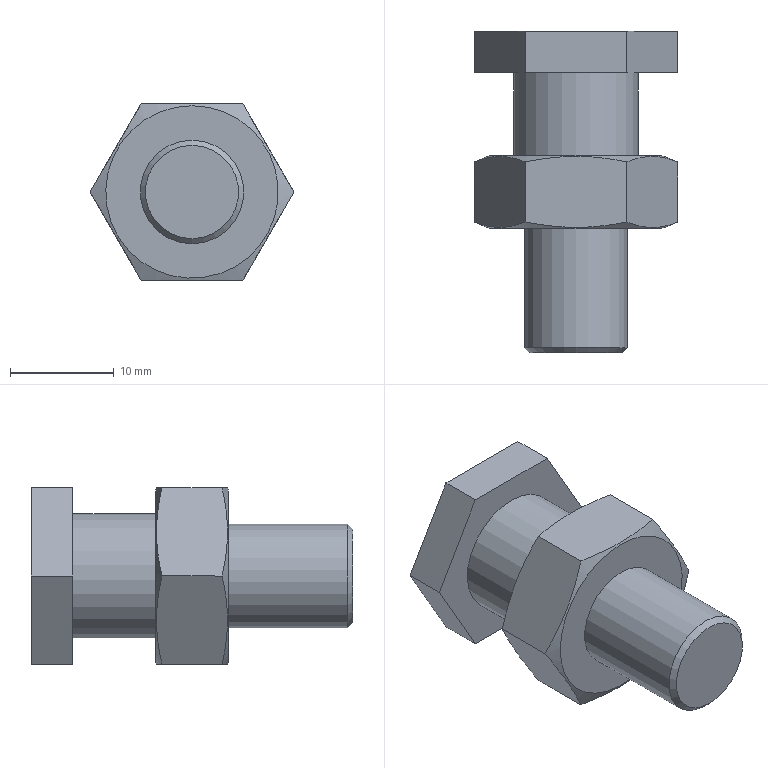Part | NX | 1 solid | 22 faces | box 19.63 x 31 x 17 mm | volume 4585 mm3 | plane 17 | cone 3 | cylinder 2 | commonest cylinder face diameters 10 x1 12 x1
STEP:
#1=CARTESIAN_POINT('',(0.,-7.,8.315));
#2=VERTEX_POINT('',#1);
#3=CARTESIAN_POINT('',(0.,-7.,0.));
#4=DIRECTION('',(0.,1.,0.));
#5=DIRECTION('',(0.,0.,1.));
#6=AXIS2_PLACEMENT_3D('',#3,#4,#5);
#7=CIRCLE('',#6,8.315);
#8=EDGE_CURVE('',#2,#2,#7,.T.);
#9=ORIENTED_EDGE('',*,*,#8,.F.);
#10=EDGE_LOOP('',(#9));
#11=FACE_BOUND('',#10,.T.);
#12=CARTESIAN_POINT('',(0.,-7.,5.));
#13=VERTEX_POINT('',#12);
#14=CARTESIAN_POINT('',(0.,-7.,0.));
#15=DIRECTION('',(0.,1.,0.));
#16=DIRECTION('',(0.,0.,1.));
#17=AXIS2_PLACEMENT_3D('',#14,#15,#16);
#18=CIRCLE('',#17,5.);
#19=EDGE_CURVE('',#13,#13,#18,.F.);
#20=ORIENTED_EDGE('',*,*,#19,.F.);
#21=EDGE_LOOP('',(#20));
#22=FACE_BOUND('',#21,.T.);
#23=CARTESIAN_POINT('',(0.,-7.,0.));
#24=DIRECTION('',(0.,1.,0.));
#25=DIRECTION('',(0.,0.,1.));
#26=AXIS2_PLACEMENT_3D('',#23,#24,#25);
#27=PLANE('',#26);
#28=ADVANCED_FACE('',(#11,#22),#27,.F.);
#29=CARTESIAN_POINT('',(4.907,-6.4,8.5));
#30=VERTEX_POINT('',#29);
#31=CARTESIAN_POINT('',(4.907,-0.6,8.5));
#32=VERTEX_POINT('',#31);
#33=CARTESIAN_POINT('',(4.907,-7.,8.5));
#34=DIRECTION('',(0.,1.,0.));
#35=VECTOR('',#34,1000.);
#36=LINE('',#33,#35);
#37=EDGE_CURVE('',#30,#32,#36,.T.);
#38=ORIENTED_EDGE('',*,*,#37,.F.);
#39=CARTESIAN_POINT('',(9.815,-6.4,0.));
#40=VERTEX_POINT('',#39);
#41=CARTESIAN_POINT('',(4.907,-6.4,8.5));
#42=CARTESIAN_POINT('',(5.721,-6.725,7.091));
#43=CARTESIAN_POINT('',(7.35,-7.126,4.27));
#44=CARTESIAN_POINT('',(9.,-6.726,1.412));
#45=CARTESIAN_POINT('',(9.815,-6.4,0.));
#46=B_SPLINE_CURVE_WITH_KNOTS('',3,(#41,#42,#43,#44,#45),.UNSPECIFIED.,.F.,.F.,(4,1,4),(0.000000232,0.004909,0.009818),.UNSPECIFIED.);
#47=EDGE_CURVE('',#30,#40,#46,.T.);
#48=ORIENTED_EDGE('',*,*,#47,.T.);
#49=CARTESIAN_POINT('',(9.815,-0.6,0.));
#50=VERTEX_POINT('',#49);
#51=CARTESIAN_POINT('',(9.815,-7.,0.));
#52=DIRECTION('',(0.,1.,0.));
#53=VECTOR('',#52,1000.);
#54=LINE('',#51,#53);
#55=EDGE_CURVE('',#40,#50,#54,.T.);
#56=ORIENTED_EDGE('',*,*,#55,.T.);
#57=CARTESIAN_POINT('',(9.815,-0.6,0.));
#58=CARTESIAN_POINT('',(9.001,-0.2746,1.409));
#59=CARTESIAN_POINT('',(7.373,0.1262,4.23));
#60=CARTESIAN_POINT('',(5.723,-0.2738,7.088));
#61=CARTESIAN_POINT('',(4.907,-0.6,8.5));
#62=B_SPLINE_CURVE_WITH_KNOTS('',3,(#57,#58,#59,#60,#61),.UNSPECIFIED.,.F.,.F.,(4,1,4),(0.000000232,0.004909,0.009818),.UNSPECIFIED.);
#63=EDGE_CURVE('',#50,#32,#62,.T.);
#64=ORIENTED_EDGE('',*,*,#63,.T.);
#65=EDGE_LOOP('',(#38,#48,#56,#64));
#66=FACE_BOUND('',#65,.T.);
#67=CARTESIAN_POINT('',(4.907,-7.,8.5));
#68=DIRECTION('',(0.866,0.,0.5));
#69=DIRECTION('',(0.5,0.,-0.866));
#70=AXIS2_PLACEMENT_3D('',#67,#68,#69);
#71=PLANE('',#70);
#72=ADVANCED_FACE('',(#66),#71,.T.);
#73=CARTESIAN_POINT('',(-4.907,-6.4,8.5));
#74=VERTEX_POINT('',#73);
#75=CARTESIAN_POINT('',(-4.907,-0.6,8.5));
#76=VERTEX_POINT('',#75);
#77=CARTESIAN_POINT('',(-4.907,-7.,8.5));
#78=DIRECTION('',(0.,1.,0.));
#79=VECTOR('',#78,1000.);
#80=LINE('',#77,#79);
#81=EDGE_CURVE('',#74,#76,#80,.T.);
#82=ORIENTED_EDGE('',*,*,#81,.F.);
#83=CARTESIAN_POINT('',(-4.907,-6.4,8.5));
#84=CARTESIAN_POINT('',(-3.285,-6.724,8.5));
#85=CARTESIAN_POINT('',(0.004586,-7.128,8.5));
#86=CARTESIAN_POINT('',(3.286,-6.724,8.5));
#87=CARTESIAN_POINT('',(4.907,-6.4,8.5));
#88=B_SPLINE_CURVE_WITH_KNOTS('',3,(#83,#84,#85,#86,#87),.UNSPECIFIED.,.F.,.F.,(4,1,4),(0.0084,0.01335,0.01831),.UNSPECIFIED.);
#89=EDGE_CURVE('',#74,#30,#88,.T.);
#90=ORIENTED_EDGE('',*,*,#89,.T.);
#91=ORIENTED_EDGE('',*,*,#37,.T.);
#92=CARTESIAN_POINT('',(-4.907,-0.6,8.5));
#93=CARTESIAN_POINT('',(-3.285,-0.2755,8.5));
#94=CARTESIAN_POINT('',(0.004586,0.1276,8.5));
#95=CARTESIAN_POINT('',(3.286,-0.2757,8.5));
#96=CARTESIAN_POINT('',(4.907,-0.6,8.5));
#97=B_SPLINE_CURVE_WITH_KNOTS('',3,(#92,#93,#94,#95,#96),.UNSPECIFIED.,.F.,.F.,(4,1,4),(0.0084,0.01335,0.01831),.UNSPECIFIED.);
#98=EDGE_CURVE('',#32,#76,#97,.F.);
#99=ORIENTED_EDGE('',*,*,#98,.T.);
#100=EDGE_LOOP('',(#82,#90,#91,#99));
#101=FACE_BOUND('',#100,.T.);
#102=CARTESIAN_POINT('',(-4.907,-7.,8.5));
#103=DIRECTION('',(0.,0.,1.));
#104=DIRECTION('',(1.,0.,0.));
#105=AXIS2_PLACEMENT_3D('',#102,#103,#104);
#106=PLANE('',#105);
#107=ADVANCED_FACE('',(#101),#106,.T.);
#108=CARTESIAN_POINT('',(-9.815,-6.4,0.));
#109=VERTEX_POINT('',#108);
#110=CARTESIAN_POINT('',(-9.815,-0.6,0.));
#111=VERTEX_POINT('',#110);
#112=CARTESIAN_POINT('',(-9.815,-7.,0.));
#113=DIRECTION('',(0.,1.,0.));
#114=VECTOR('',#113,1000.);
#115=LINE('',#112,#114);
#116=EDGE_CURVE('',#109,#111,#115,.T.);
#117=ORIENTED_EDGE('',*,*,#116,.F.);
#118=CARTESIAN_POINT('',(-9.815,-6.4,0.));
#119=CARTESIAN_POINT('',(-9.001,-6.725,1.409));
#120=CARTESIAN_POINT('',(-7.373,-7.126,4.23));
#121=CARTESIAN_POINT('',(-5.723,-6.726,7.088));
#122=CARTESIAN_POINT('',(-4.907,-6.4,8.5));
#123=B_SPLINE_CURVE_WITH_KNOTS('',3,(#118,#119,#120,#121,#122),.UNSPECIFIED.,.F.,.F.,(4,1,4),(0.000000232,0.004909,0.009818),.UNSPECIFIED.);
#124=EDGE_CURVE('',#109,#74,#123,.T.);
#125=ORIENTED_EDGE('',*,*,#124,.T.);
#126=ORIENTED_EDGE('',*,*,#81,.T.);
#127=CARTESIAN_POINT('',(-4.907,-0.6,8.5));
#128=CARTESIAN_POINT('',(-5.721,-0.2746,7.091));
#129=CARTESIAN_POINT('',(-7.35,0.1262,4.27));
#130=CARTESIAN_POINT('',(-9.,-0.2738,1.412));
#131=CARTESIAN_POINT('',(-9.815,-0.6,0.));
#132=B_SPLINE_CURVE_WITH_KNOTS('',3,(#127,#128,#129,#130,#131),.UNSPECIFIED.,.F.,.F.,(4,1,4),(0.000000232,0.004909,0.009818),.UNSPECIFIED.);
#133=EDGE_CURVE('',#76,#111,#132,.T.);
#134=ORIENTED_EDGE('',*,*,#133,.T.);
#135=EDGE_LOOP('',(#117,#125,#126,#134));
#136=FACE_BOUND('',#135,.T.);
#137=CARTESIAN_POINT('',(-9.815,-7.,0.));
#138=DIRECTION('',(-0.866,0.,0.5));
#139=DIRECTION('',(0.5,0.,0.866));
#140=AXIS2_PLACEMENT_3D('',#137,#138,#139);
#141=PLANE('',#140);
#142=ADVANCED_FACE('',(#136),#141,.T.);
#143=CARTESIAN_POINT('',(-4.907,-6.4,-8.5));
#144=VERTEX_POINT('',#143);
#145=CARTESIAN_POINT('',(-4.907,-0.6,-8.5));
#146=VERTEX_POINT('',#145);
#147=CARTESIAN_POINT('',(-4.907,-7.,-8.5));
#148=DIRECTION('',(0.,1.,0.));
#149=VECTOR('',#148,1000.);
#150=LINE('',#147,#149);
#151=EDGE_CURVE('',#144,#146,#150,.T.);
#152=ORIENTED_EDGE('',*,*,#151,.F.);
#153=CARTESIAN_POINT('',(-4.907,-6.4,-8.5));
#154=CARTESIAN_POINT('',(-5.721,-6.725,-7.091));
#155=CARTESIAN_POINT('',(-7.35,-7.126,-4.27));
#156=CARTESIAN_POINT('',(-9.,-6.726,-1.412));
#157=CARTESIAN_POINT('',(-9.815,-6.4,0.));
#158=B_SPLINE_CURVE_WITH_KNOTS('',3,(#153,#154,#155,#156,#157),.UNSPECIFIED.,.F.,.F.,(4,1,4),(0.000000232,0.004909,0.009818),.UNSPECIFIED.);
#159=EDGE_CURVE('',#144,#109,#158,.T.);
#160=ORIENTED_EDGE('',*,*,#159,.T.);
#161=ORIENTED_EDGE('',*,*,#116,.T.);
#162=CARTESIAN_POINT('',(-9.815,-0.6,0.));
#163=CARTESIAN_POINT('',(-9.001,-0.2746,-1.409));
#164=CARTESIAN_POINT('',(-7.373,0.1262,-4.23));
#165=CARTESIAN_POINT('',(-5.723,-0.2738,-7.088));
#166=CARTESIAN_POINT('',(-4.907,-0.6,-8.5));
#167=B_SPLINE_CURVE_WITH_KNOTS('',3,(#162,#163,#164,#165,#166),.UNSPECIFIED.,.F.,.F.,(4,1,4),(0.000000232,0.004909,0.009818),.UNSPECIFIED.);
#168=EDGE_CURVE('',#111,#146,#167,.T.);
#169=ORIENTED_EDGE('',*,*,#168,.T.);
#170=EDGE_LOOP('',(#152,#160,#161,#169));
#171=FACE_BOUND('',#170,.T.);
#172=CARTESIAN_POINT('',(-4.907,-7.,-8.5));
#173=DIRECTION('',(-0.866,0.,-0.5));
#174=DIRECTION('',(-0.5,0.,0.866));
#175=AXIS2_PLACEMENT_3D('',#172,#173,#174);
#176=PLANE('',#175);
#177=ADVANCED_FACE('',(#171),#176,.T.);
#178=CARTESIAN_POINT('',(4.907,-6.4,-8.5));
#179=VERTEX_POINT('',#178);
#180=CARTESIAN_POINT('',(4.907,-0.6,-8.5));
#181=VERTEX_POINT('',#180);
#182=CARTESIAN_POINT('',(4.907,-7.,-8.5));
#183=DIRECTION('',(0.,1.,0.));
#184=VECTOR('',#183,1000.);
#185=LINE('',#182,#184);
#186=EDGE_CURVE('',#179,#181,#185,.T.);
#187=ORIENTED_EDGE('',*,*,#186,.F.);
#188=CARTESIAN_POINT('',(-4.907,-6.4,-8.5));
#189=CARTESIAN_POINT('',(-3.285,-6.724,-8.5));
#190=CARTESIAN_POINT('',(0.004586,-7.128,-8.5));
#191=CARTESIAN_POINT('',(3.286,-6.724,-8.5));
#192=CARTESIAN_POINT('',(4.907,-6.4,-8.5));
#193=B_SPLINE_CURVE_WITH_KNOTS('',3,(#188,#189,#190,#191,#192),.UNSPECIFIED.,.F.,.F.,(4,1,4),(0.0084,0.01335,0.01831),.UNSPECIFIED.);
#194=EDGE_CURVE('',#179,#144,#193,.F.);
#195=ORIENTED_EDGE('',*,*,#194,.T.);
#196=ORIENTED_EDGE('',*,*,#151,.T.);
#197=CARTESIAN_POINT('',(-4.907,-0.6,-8.5));
#198=CARTESIAN_POINT('',(-3.285,-0.2755,-8.5));
#199=CARTESIAN_POINT('',(0.004586,0.1276,-8.5));
#200=CARTESIAN_POINT('',(3.286,-0.2757,-8.5));
#201=CARTESIAN_POINT('',(4.907,-0.6,-8.5));
#202=B_SPLINE_CURVE_WITH_KNOTS('',3,(#197,#198,#199,#200,#201),.UNSPECIFIED.,.F.,.F.,(4,1,4),(0.0084,0.01335,0.01831),.UNSPECIFIED.);
#203=EDGE_CURVE('',#146,#181,#202,.T.);
#204=ORIENTED_EDGE('',*,*,#203,.T.);
#205=EDGE_LOOP('',(#187,#195,#196,#204));
#206=FACE_BOUND('',#205,.T.);
#207=CARTESIAN_POINT('',(4.907,-7.,-8.5));
#208=DIRECTION('',(0.,0.,-1.));
#209=DIRECTION('',(-1.,0.,0.));
#210=AXIS2_PLACEMENT_3D('',#207,#208,#209);
#211=PLANE('',#210);
#212=ADVANCED_FACE('',(#206),#211,.T.);
#213=ORIENTED_EDGE('',*,*,#55,.F.);
#214=CARTESIAN_POINT('',(9.815,-6.4,0.));
#215=CARTESIAN_POINT('',(9.001,-6.725,-1.409));
#216=CARTESIAN_POINT('',(7.373,-7.126,-4.23));
#217=CARTESIAN_POINT('',(5.723,-6.726,-7.088));
#218=CARTESIAN_POINT('',(4.907,-6.4,-8.5));
#219=B_SPLINE_CURVE_WITH_KNOTS('',3,(#214,#215,#216,#217,#218),.UNSPECIFIED.,.F.,.F.,(4,1,4),(0.000000232,0.004909,0.009818),.UNSPECIFIED.);
#220=EDGE_CURVE('',#40,#179,#219,.T.);
#221=ORIENTED_EDGE('',*,*,#220,.T.);
#222=ORIENTED_EDGE('',*,*,#186,.T.);
#223=CARTESIAN_POINT('',(4.907,-0.6,-8.5));
#224=CARTESIAN_POINT('',(5.721,-0.2746,-7.091));
#225=CARTESIAN_POINT('',(7.35,0.1262,-4.27));
#226=CARTESIAN_POINT('',(9.,-0.2738,-1.412));
#227=CARTESIAN_POINT('',(9.815,-0.6,0.));
#228=B_SPLINE_CURVE_WITH_KNOTS('',3,(#223,#224,#225,#226,#227),.UNSPECIFIED.,.F.,.F.,(4,1,4),(0.000000232,0.004909,0.009818),.UNSPECIFIED.);
#229=EDGE_CURVE('',#181,#50,#228,.T.);
#230=ORIENTED_EDGE('',*,*,#229,.T.);
#231=EDGE_LOOP('',(#213,#221,#222,#230));
#232=FACE_BOUND('',#231,.T.);
#233=CARTESIAN_POINT('',(9.815,-7.,0.));
#234=DIRECTION('',(0.866,0.,-0.5));
#235=DIRECTION('',(-0.5,0.,-0.866));
#236=AXIS2_PLACEMENT_3D('',#233,#234,#235);
#237=PLANE('',#236);
#238=ADVANCED_FACE('',(#232),#237,.T.);
#239=CARTESIAN_POINT('',(0.,0.,6.));
#240=VERTEX_POINT('',#239);
#241=CARTESIAN_POINT('',(0.,0.,0.));
#242=DIRECTION('',(0.,1.,0.));
#243=DIRECTION('',(0.,0.,1.));
#244=AXIS2_PLACEMENT_3D('',#241,#242,#243);
#245=CIRCLE('',#244,6.);
#246=EDGE_CURVE('',#240,#240,#245,.T.);
#247=ORIENTED_EDGE('',*,*,#246,.F.);
#248=EDGE_LOOP('',(#247));
#249=FACE_BOUND('',#248,.T.);
#250=CARTESIAN_POINT('',(0.,0.,8.315));
#251=VERTEX_POINT('',#250);
#252=CARTESIAN_POINT('',(0.,0.,0.));
#253=DIRECTION('',(0.,1.,0.));
#254=DIRECTION('',(0.,0.,1.));
#255=AXIS2_PLACEMENT_3D('',#252,#253,#254);
#256=CIRCLE('',#255,8.315);
#257=EDGE_CURVE('',#251,#251,#256,.T.);
#258=ORIENTED_EDGE('',*,*,#257,.T.);
#259=EDGE_LOOP('',(#258));
#260=FACE_BOUND('',#259,.T.);
#261=CARTESIAN_POINT('',(0.,0.,0.));
#262=DIRECTION('',(0.,1.,0.));
#263=DIRECTION('',(0.,0.,1.));
#264=AXIS2_PLACEMENT_3D('',#261,#262,#263);
#265=PLANE('',#264);
#266=ADVANCED_FACE('',(#249,#260),#265,.T.);
#267=CARTESIAN_POINT('',(4.907,8.,8.5));
#268=VERTEX_POINT('',#267);
#269=CARTESIAN_POINT('',(9.815,8.,0.));
#270=VERTEX_POINT('',#269);
#271=CARTESIAN_POINT('',(4.907,8.,8.5));
#272=DIRECTION('',(0.5,0.,-0.866));
#273=VECTOR('',#272,1000.);
#274=LINE('',#271,#273);
#275=EDGE_CURVE('',#268,#270,#274,.T.);
#276=ORIENTED_EDGE('',*,*,#275,.T.);
#277=CARTESIAN_POINT('',(9.815,12.,0.));
#278=VERTEX_POINT('',#277);
#279=CARTESIAN_POINT('',(9.815,-7.,0.));
#280=DIRECTION('',(0.,1.,0.));
#281=VECTOR('',#280,1000.);
#282=LINE('',#279,#281);
#283=EDGE_CURVE('',#270,#278,#282,.T.);
#284=ORIENTED_EDGE('',*,*,#283,.T.);
#285=CARTESIAN_POINT('',(4.907,12.,8.5));
#286=VERTEX_POINT('',#285);
#287=CARTESIAN_POINT('',(4.907,12.,8.5));
#288=DIRECTION('',(0.5,0.,-0.866));
#289=VECTOR('',#288,1000.);
#290=LINE('',#287,#289);
#291=EDGE_CURVE('',#286,#278,#290,.T.);
#292=ORIENTED_EDGE('',*,*,#291,.F.);
#293=CARTESIAN_POINT('',(4.907,-7.,8.5));
#294=DIRECTION('',(0.,1.,0.));
#295=VECTOR('',#294,1000.);
#296=LINE('',#293,#295);
#297=EDGE_CURVE('',#268,#286,#296,.T.);
#298=ORIENTED_EDGE('',*,*,#297,.F.);
#299=EDGE_LOOP('',(#276,#284,#292,#298));
#300=FACE_BOUND('',#299,.T.);
#301=CARTESIAN_POINT('',(4.907,-7.,8.5));
#302=DIRECTION('',(0.866,0.,0.5));
#303=DIRECTION('',(0.5,0.,-0.866));
#304=AXIS2_PLACEMENT_3D('',#301,#302,#303);
#305=PLANE('',#304);
#306=ADVANCED_FACE('',(#300),#305,.T.);
#307=CARTESIAN_POINT('',(-4.907,8.,8.5));
#308=VERTEX_POINT('',#307);
#309=CARTESIAN_POINT('',(-4.907,8.,8.5));
#310=DIRECTION('',(1.,0.,0.));
#311=VECTOR('',#310,1000.);
#312=LINE('',#309,#311);
#313=EDGE_CURVE('',#308,#268,#312,.T.);
#314=ORIENTED_EDGE('',*,*,#313,.T.);
#315=ORIENTED_EDGE('',*,*,#297,.T.);
#316=CARTESIAN_POINT('',(-4.907,12.,8.5));
#317=VERTEX_POINT('',#316);
#318=CARTESIAN_POINT('',(-4.907,12.,8.5));
#319=DIRECTION('',(1.,0.,0.));
#320=VECTOR('',#319,1000.);
#321=LINE('',#318,#320);
#322=EDGE_CURVE('',#317,#286,#321,.T.);
#323=ORIENTED_EDGE('',*,*,#322,.F.);
#324=CARTESIAN_POINT('',(-4.907,-7.,8.5));
#325=DIRECTION('',(0.,1.,0.));
#326=VECTOR('',#325,1000.);
#327=LINE('',#324,#326);
#328=EDGE_CURVE('',#308,#317,#327,.T.);
#329=ORIENTED_EDGE('',*,*,#328,.F.);
#330=EDGE_LOOP('',(#314,#315,#323,#329));
#331=FACE_BOUND('',#330,.T.);
#332=CARTESIAN_POINT('',(-4.907,-7.,8.5));
#333=DIRECTION('',(0.,0.,1.));
#334=DIRECTION('',(1.,0.,0.));
#335=AXIS2_PLACEMENT_3D('',#332,#333,#334);
#336=PLANE('',#335);
#337=ADVANCED_FACE('',(#331),#336,.T.);
#338=CARTESIAN_POINT('',(-9.815,8.,0.));
#339=VERTEX_POINT('',#338);
#340=CARTESIAN_POINT('',(-9.815,8.,0.));
#341=DIRECTION('',(0.5,0.,0.866));
#342=VECTOR('',#341,1000.);
#343=LINE('',#340,#342);
#344=EDGE_CURVE('',#339,#308,#343,.T.);
#345=ORIENTED_EDGE('',*,*,#344,.T.);
#346=ORIENTED_EDGE('',*,*,#328,.T.);
#347=CARTESIAN_POINT('',(-9.815,12.,0.));
#348=VERTEX_POINT('',#347);
#349=CARTESIAN_POINT('',(-9.815,12.,0.));
#350=DIRECTION('',(0.5,0.,0.866));
#351=VECTOR('',#350,1000.);
#352=LINE('',#349,#351);
#353=EDGE_CURVE('',#348,#317,#352,.T.);
#354=ORIENTED_EDGE('',*,*,#353,.F.);
#355=CARTESIAN_POINT('',(-9.815,-7.,0.));
#356=DIRECTION('',(0.,1.,0.));
#357=VECTOR('',#356,1000.);
#358=LINE('',#355,#357);
#359=EDGE_CURVE('',#339,#348,#358,.T.);
#360=ORIENTED_EDGE('',*,*,#359,.F.);
#361=EDGE_LOOP('',(#345,#346,#354,#360));
#362=FACE_BOUND('',#361,.T.);
#363=CARTESIAN_POINT('',(-9.815,-7.,0.));
#364=DIRECTION('',(-0.866,0.,0.5));
#365=DIRECTION('',(0.5,0.,0.866));
#366=AXIS2_PLACEMENT_3D('',#363,#364,#365);
#367=PLANE('',#366);
#368=ADVANCED_FACE('',(#362),#367,.T.);
#369=CARTESIAN_POINT('',(-4.907,8.,-8.5));
#370=VERTEX_POINT('',#369);
#371=CARTESIAN_POINT('',(-4.907,8.,-8.5));
#372=DIRECTION('',(-0.5,0.,0.866));
#373=VECTOR('',#372,1000.);
#374=LINE('',#371,#373);
#375=EDGE_CURVE('',#370,#339,#374,.T.);
#376=ORIENTED_EDGE('',*,*,#375,.T.);
#377=ORIENTED_EDGE('',*,*,#359,.T.);
#378=CARTESIAN_POINT('',(-4.907,12.,-8.5));
#379=VERTEX_POINT('',#378);
#380=CARTESIAN_POINT('',(-4.907,12.,-8.5));
#381=DIRECTION('',(-0.5,0.,0.866));
#382=VECTOR('',#381,1000.);
#383=LINE('',#380,#382);
#384=EDGE_CURVE('',#379,#348,#383,.T.);
#385=ORIENTED_EDGE('',*,*,#384,.F.);
#386=CARTESIAN_POINT('',(-4.907,-7.,-8.5));
#387=DIRECTION('',(0.,1.,0.));
#388=VECTOR('',#387,1000.);
#389=LINE('',#386,#388);
#390=EDGE_CURVE('',#370,#379,#389,.T.);
#391=ORIENTED_EDGE('',*,*,#390,.F.);
#392=EDGE_LOOP('',(#376,#377,#385,#391));
#393=FACE_BOUND('',#392,.T.);
#394=CARTESIAN_POINT('',(-4.907,-7.,-8.5));
#395=DIRECTION('',(-0.866,0.,-0.5));
#396=DIRECTION('',(-0.5,0.,0.866));
#397=AXIS2_PLACEMENT_3D('',#394,#395,#396);
#398=PLANE('',#397);
#399=ADVANCED_FACE('',(#393),#398,.T.);
#400=CARTESIAN_POINT('',(4.907,8.,-8.5));
#401=VERTEX_POINT('',#400);
#402=CARTESIAN_POINT('',(4.907,8.,-8.5));
#403=DIRECTION('',(-1.,0.,0.));
#404=VECTOR('',#403,1000.);
#405=LINE('',#402,#404);
#406=EDGE_CURVE('',#401,#370,#405,.T.);
#407=ORIENTED_EDGE('',*,*,#406,.T.);
#408=ORIENTED_EDGE('',*,*,#390,.T.);
#409=CARTESIAN_POINT('',(4.907,12.,-8.5));
#410=VERTEX_POINT('',#409);
#411=CARTESIAN_POINT('',(4.907,12.,-8.5));
#412=DIRECTION('',(-1.,0.,0.));
#413=VECTOR('',#412,1000.);
#414=LINE('',#411,#413);
#415=EDGE_CURVE('',#410,#379,#414,.T.);
#416=ORIENTED_EDGE('',*,*,#415,.F.);
#417=CARTESIAN_POINT('',(4.907,-7.,-8.5));
#418=DIRECTION('',(0.,1.,0.));
#419=VECTOR('',#418,1000.);
#420=LINE('',#417,#419);
#421=EDGE_CURVE('',#401,#410,#420,.T.);
#422=ORIENTED_EDGE('',*,*,#421,.F.);
#423=EDGE_LOOP('',(#407,#408,#416,#422));
#424=FACE_BOUND('',#423,.T.);
#425=CARTESIAN_POINT('',(4.907,-7.,-8.5));
#426=DIRECTION('',(0.,0.,-1.));
#427=DIRECTION('',(-1.,0.,0.));
#428=AXIS2_PLACEMENT_3D('',#425,#426,#427);
#429=PLANE('',#428);
#430=ADVANCED_FACE('',(#424),#429,.T.);
#431=CARTESIAN_POINT('',(9.815,8.,0.));
#432=DIRECTION('',(-0.5,0.,-0.866));
#433=VECTOR('',#432,1000.);
#434=LINE('',#431,#433);
#435=EDGE_CURVE('',#270,#401,#434,.T.);
#436=ORIENTED_EDGE('',*,*,#435,.T.);
#437=ORIENTED_EDGE('',*,*,#421,.T.);
#438=CARTESIAN_POINT('',(9.815,12.,0.));
#439=DIRECTION('',(-0.5,0.,-0.866));
#440=VECTOR('',#439,1000.);
#441=LINE('',#438,#440);
#442=EDGE_CURVE('',#278,#410,#441,.T.);
#443=ORIENTED_EDGE('',*,*,#442,.F.);
#444=ORIENTED_EDGE('',*,*,#283,.F.);
#445=EDGE_LOOP('',(#436,#437,#443,#444));
#446=FACE_BOUND('',#445,.T.);
#447=CARTESIAN_POINT('',(9.815,-7.,0.));
#448=DIRECTION('',(0.866,0.,-0.5));
#449=DIRECTION('',(-0.5,0.,-0.866));
#450=AXIS2_PLACEMENT_3D('',#447,#448,#449);
#451=PLANE('',#450);
#452=ADVANCED_FACE('',(#446),#451,.T.);
#453=ORIENTED_EDGE('',*,*,#291,.T.);
#454=ORIENTED_EDGE('',*,*,#442,.T.);
#455=ORIENTED_EDGE('',*,*,#415,.T.);
#456=ORIENTED_EDGE('',*,*,#384,.T.);
#457=ORIENTED_EDGE('',*,*,#353,.T.);
#458=ORIENTED_EDGE('',*,*,#322,.T.);
#459=EDGE_LOOP('',(#453,#454,#455,#456,#457,#458));
#460=FACE_BOUND('',#459,.T.);
#461=CARTESIAN_POINT('',(0.,12.,0.));
#462=DIRECTION('',(0.,1.,0.));
#463=DIRECTION('',(0.,0.,1.));
#464=AXIS2_PLACEMENT_3D('',#461,#462,#463);
#465=PLANE('',#464);
#466=ADVANCED_FACE('',(#460),#465,.T.);
#467=ORIENTED_EDGE('',*,*,#313,.F.);
#468=ORIENTED_EDGE('',*,*,#344,.F.);
#469=ORIENTED_EDGE('',*,*,#375,.F.);
#470=ORIENTED_EDGE('',*,*,#406,.F.);
#471=ORIENTED_EDGE('',*,*,#435,.F.);
#472=ORIENTED_EDGE('',*,*,#275,.F.);
#473=EDGE_LOOP('',(#467,#468,#469,#470,#471,#472));
#474=FACE_BOUND('',#473,.T.);
#475=CARTESIAN_POINT('',(0.,8.,6.));
#476=VERTEX_POINT('',#475);
#477=CARTESIAN_POINT('',(0.,8.,0.));
#478=DIRECTION('',(0.,1.,0.));
#479=DIRECTION('',(0.,0.,1.));
#480=AXIS2_PLACEMENT_3D('',#477,#478,#479);
#481=CIRCLE('',#480,6.);
#482=EDGE_CURVE('',#476,#476,#481,.T.);
#483=ORIENTED_EDGE('',*,*,#482,.T.);
#484=EDGE_LOOP('',(#483));
#485=FACE_BOUND('',#484,.T.);
#486=CARTESIAN_POINT('',(0.,8.,0.));
#487=DIRECTION('',(0.,1.,0.));
#488=DIRECTION('',(0.,0.,1.));
#489=AXIS2_PLACEMENT_3D('',#486,#487,#488);
#490=PLANE('',#489);
#491=ADVANCED_FACE('',(#474,#485),#490,.F.);
#492=ORIENTED_EDGE('',*,*,#482,.F.);
#493=EDGE_LOOP('',(#492));
#494=FACE_BOUND('',#493,.T.);
#495=ORIENTED_EDGE('',*,*,#246,.T.);
#496=EDGE_LOOP('',(#495));
#497=FACE_BOUND('',#496,.T.);
#498=CARTESIAN_POINT('',(0.,8.,0.));
#499=DIRECTION('',(0.,-1.,0.));
#500=DIRECTION('',(0.,0.,-1.));
#501=AXIS2_PLACEMENT_3D('',#498,#499,#500);
#502=CYLINDRICAL_SURFACE('',#501,6.);
#503=ADVANCED_FACE('',(#494,#497),#502,.T.);
#504=ORIENTED_EDGE('',*,*,#203,.F.);
#505=ORIENTED_EDGE('',*,*,#168,.F.);
#506=ORIENTED_EDGE('',*,*,#133,.F.);
#507=ORIENTED_EDGE('',*,*,#98,.F.);
#508=ORIENTED_EDGE('',*,*,#63,.F.);
#509=ORIENTED_EDGE('',*,*,#229,.F.);
#510=EDGE_LOOP('',(#504,#505,#506,#507,#508,#509));
#511=FACE_BOUND('',#510,.T.);
#512=ORIENTED_EDGE('',*,*,#257,.F.);
#513=EDGE_LOOP('',(#512));
#514=FACE_BOUND('',#513,.T.);
#515=CARTESIAN_POINT('',(0.,0.,0.));
#516=DIRECTION('',(0.,-1.,0.));
#517=DIRECTION('',(0.,0.,-1.));
#518=AXIS2_PLACEMENT_3D('',#515,#516,#517);
#519=CONICAL_SURFACE('',#518,8.315,1.19);
#520=ADVANCED_FACE('',(#511,#514),#519,.T.);
#521=ORIENTED_EDGE('',*,*,#89,.F.);
#522=ORIENTED_EDGE('',*,*,#124,.F.);
#523=ORIENTED_EDGE('',*,*,#159,.F.);
#524=ORIENTED_EDGE('',*,*,#194,.F.);
#525=ORIENTED_EDGE('',*,*,#220,.F.);
#526=ORIENTED_EDGE('',*,*,#47,.F.);
#527=EDGE_LOOP('',(#521,#522,#523,#524,#525,#526));
#528=FACE_BOUND('',#527,.T.);
#529=ORIENTED_EDGE('',*,*,#8,.T.);
#530=EDGE_LOOP('',(#529));
#531=FACE_BOUND('',#530,.T.);
#532=CARTESIAN_POINT('',(0.,-7.,0.));
#533=DIRECTION('',(0.,1.,0.));
#534=DIRECTION('',(0.,0.,-1.));
#535=AXIS2_PLACEMENT_3D('',#532,#533,#534);
#536=CONICAL_SURFACE('',#535,8.315,1.19);
#537=ADVANCED_FACE('',(#528,#531),#536,.T.);
#538=CARTESIAN_POINT('',(0.,-18.5,-5.));
#539=VERTEX_POINT('',#538);
#540=CARTESIAN_POINT('',(0.,-18.5,0.));
#541=DIRECTION('',(0.,-1.,0.));
#542=DIRECTION('',(0.,0.,-1.));
#543=AXIS2_PLACEMENT_3D('',#540,#541,#542);
#544=CIRCLE('',#543,5.);
#545=EDGE_CURVE('',#539,#539,#544,.F.);
#546=ORIENTED_EDGE('',*,*,#545,.T.);
#547=EDGE_LOOP('',(#546));
#548=FACE_BOUND('',#547,.T.);
#549=ORIENTED_EDGE('',*,*,#19,.T.);
#550=EDGE_LOOP('',(#549));
#551=FACE_BOUND('',#550,.T.);
#552=CARTESIAN_POINT('',(0.,-19.,0.));
#553=DIRECTION('',(0.,1.,0.));
#554=DIRECTION('',(0.,0.,1.));
#555=AXIS2_PLACEMENT_3D('',#552,#553,#554);
#556=CYLINDRICAL_SURFACE('',#555,5.);
#557=ADVANCED_FACE('',(#548,#551),#556,.T.);
#558=CARTESIAN_POINT('',(0.,-19.,-4.5));
#559=VERTEX_POINT('',#558);
#560=CARTESIAN_POINT('',(0.,-19.,0.));
#561=DIRECTION('',(0.,-1.,0.));
#562=DIRECTION('',(0.,0.,-1.));
#563=AXIS2_PLACEMENT_3D('',#560,#561,#562);
#564=CIRCLE('',#563,4.5);
#565=EDGE_CURVE('',#559,#559,#564,.T.);
#566=ORIENTED_EDGE('',*,*,#565,.T.);
#567=EDGE_LOOP('',(#566));
#568=FACE_BOUND('',#567,.T.);
#569=CARTESIAN_POINT('',(0.,-19.,0.));
#570=DIRECTION('',(0.,-1.,0.));
#571=DIRECTION('',(0.,0.,-1.));
#572=AXIS2_PLACEMENT_3D('',#569,#570,#571);
#573=PLANE('',#572);
#574=ADVANCED_FACE('',(#568),#573,.T.);
#575=ORIENTED_EDGE('',*,*,#545,.F.);
#576=EDGE_LOOP('',(#575));
#577=FACE_BOUND('',#576,.T.);
#578=ORIENTED_EDGE('',*,*,#565,.F.);
#579=EDGE_LOOP('',(#578));
#580=FACE_BOUND('',#579,.T.);
#581=CARTESIAN_POINT('',(0.,-19.,0.));
#582=DIRECTION('',(0.,1.,0.));
#583=DIRECTION('',(0.,0.,1.));
#584=AXIS2_PLACEMENT_3D('',#581,#582,#583);
#585=CONICAL_SURFACE('',#584,4.5,0.7854);
#586=ADVANCED_FACE('',(#577,#580),#585,.T.);
#587=CLOSED_SHELL('',(#28,#72,#107,#142,#177,#212,#238,#266,#306,#337,#368,#399,#430,#452,#466,#491,#503,#520,#537,#557,#574,#586));
#588=MANIFOLD_SOLID_BREP('',#587);
#589=(LENGTH_UNIT()NAMED_UNIT(*)SI_UNIT(.MILLI.,.METRE.));
#590=UNCERTAINTY_MEASURE_WITH_UNIT(LENGTH_MEASURE(0.0508),#589,'','');
#591=(NAMED_UNIT(*)PLANE_ANGLE_UNIT()SI_UNIT($,.RADIAN.));
#592=(NAMED_UNIT(*)SI_UNIT($,.STERADIAN.)SOLID_ANGLE_UNIT());
#593=(GEOMETRIC_REPRESENTATION_CONTEXT(3)GLOBAL_UNCERTAINTY_ASSIGNED_CONTEXT((#590))GLOBAL_UNIT_ASSIGNED_CONTEXT((#589,#591,#592))REPRESENTATION_CONTEXT('',''));
#594=ADVANCED_BREP_SHAPE_REPRESENTATION('',(#588),#593);